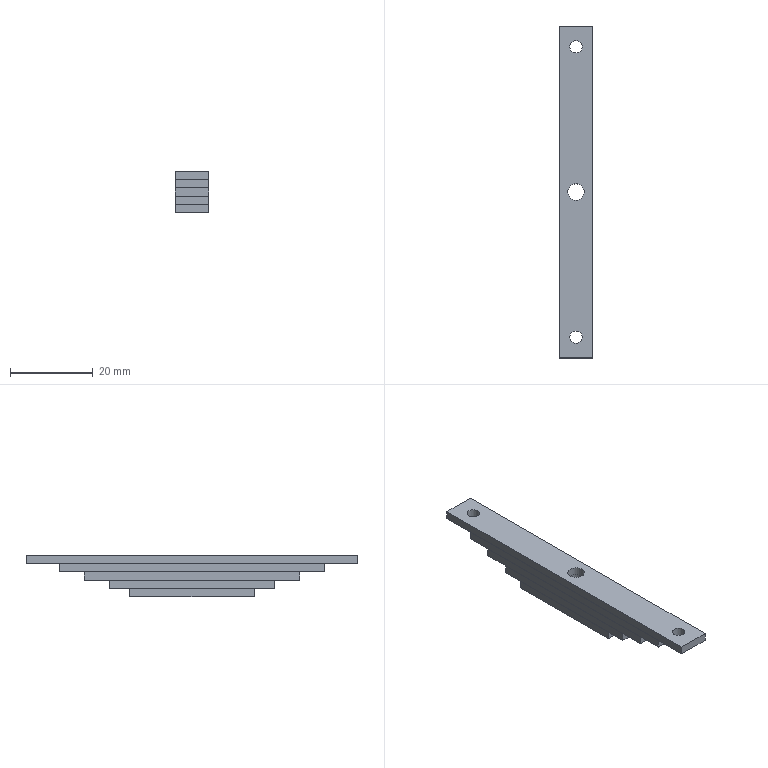Part | STEP file | 1-54.1 | 5 solids | 37 faces | box 8 x 80 x 10 mm | volume 4102 mm3 | plane 30 | cylinder 7 | commonest cylinder face diameters 4 x5 3 x2